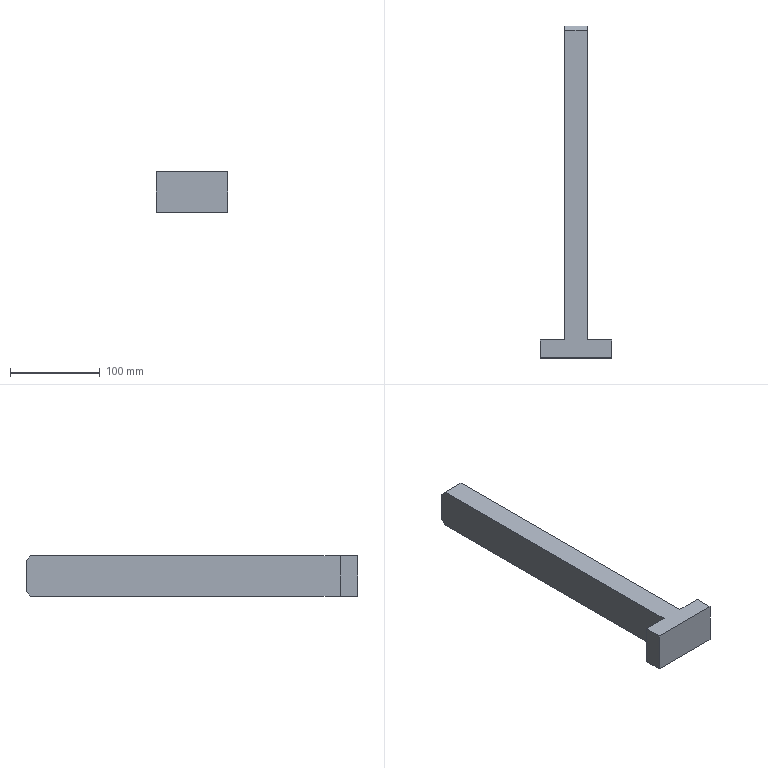Part | STEP file | 2012-06-08-018 | 1 solid | 12 faces | box 80 x 370 x 45 mm | volume 465125 mm3 | plane 12
STEP:
#1=CARTESIAN_POINT('',(0.,0.,0.));
#2=DIRECTION('',(0.,0.,1.));
#3=DIRECTION('',(1.,0.,0.));
#4=AXIS2_PLACEMENT_3D('',#1,#2,#3);
#5=CARTESIAN_POINT('',(0.,20.,0.));
#6=VERTEX_POINT('',#5);
#7=CARTESIAN_POINT('',(0.,0.,0.));
#8=VERTEX_POINT('',#7);
#9=CARTESIAN_POINT('',(0.,0.,0.));
#10=DIRECTION('',(0.,-1.,0.));
#11=VECTOR('',#10,1.);
#12=LINE('',#9,#11);
#13=CARTESIAN_POINT('',(0.,0.,45.));
#14=DIRECTION('',(1.,0.,0.));
#15=DIRECTION('',(0.,0.,-1.));
#16=AXIS2_PLACEMENT_3D('',#13,#14,#15);
#17=PLANE('',#16);
#18=CARTESIAN_POINT('',(45.,0.));
#19=DIRECTION('',(0.,-1.));
#20=VECTOR('',#19,1.);
#21=LINE('',#18,#20);
#22=(GEOMETRIC_REPRESENTATION_CONTEXT(2)PARAMETRIC_REPRESENTATION_CONTEXT()REPRESENTATION_CONTEXT('',''));
#23=DEFINITIONAL_REPRESENTATION('',(#21),#22);
#24=PCURVE('',#17,#23);
#25=CARTESIAN_POINT('',(0.,20.,0.));
#26=DIRECTION('',(0.,0.,-1.));
#27=DIRECTION('',(-1.,0.,0.));
#28=AXIS2_PLACEMENT_3D('',#25,#26,#27);
#29=PLANE('',#28);
#30=CARTESIAN_POINT('',(0.,-20.));
#31=DIRECTION('',(0.,-1.));
#32=VECTOR('',#31,1.);
#33=LINE('',#30,#32);
#34=(GEOMETRIC_REPRESENTATION_CONTEXT(2)PARAMETRIC_REPRESENTATION_CONTEXT()REPRESENTATION_CONTEXT('',''));
#35=DEFINITIONAL_REPRESENTATION('',(#33),#34);
#36=PCURVE('',#29,#35);
#37=SURFACE_CURVE('',#12,(#24,#36),.PCURVE_S1.);
#38=EDGE_CURVE('',#6,#8,#37,.T.);
#39=ORIENTED_EDGE('',*,*,#38,.T.);
#40=CARTESIAN_POINT('',(0.,0.,45.));
#41=VERTEX_POINT('',#40);
#42=CARTESIAN_POINT('',(0.,0.,45.));
#43=DIRECTION('',(0.,0.,-1.));
#44=VECTOR('',#43,1.);
#45=LINE('',#42,#44);
#46=CARTESIAN_POINT('',(0.,0.));
#47=DIRECTION('',(1.,0.));
#48=VECTOR('',#47,1.);
#49=LINE('',#46,#48);
#50=(GEOMETRIC_REPRESENTATION_CONTEXT(2)PARAMETRIC_REPRESENTATION_CONTEXT()REPRESENTATION_CONTEXT('',''));
#51=DEFINITIONAL_REPRESENTATION('',(#49),#50);
#52=PCURVE('',#17,#51);
#53=CARTESIAN_POINT('',(0.,0.,45.));
#54=DIRECTION('',(0.,1.,0.));
#55=DIRECTION('',(0.,0.,1.));
#56=AXIS2_PLACEMENT_3D('',#53,#54,#55);
#57=PLANE('',#56);
#58=CARTESIAN_POINT('',(0.,0.));
#59=DIRECTION('',(-1.,0.));
#60=VECTOR('',#59,1.);
#61=LINE('',#58,#60);
#62=(GEOMETRIC_REPRESENTATION_CONTEXT(2)PARAMETRIC_REPRESENTATION_CONTEXT()REPRESENTATION_CONTEXT('',''));
#63=DEFINITIONAL_REPRESENTATION('',(#61),#62);
#64=PCURVE('',#57,#63);
#65=SURFACE_CURVE('',#45,(#52,#64),.PCURVE_S1.);
#66=EDGE_CURVE('',#41,#8,#65,.T.);
#67=ORIENTED_EDGE('',*,*,#66,.F.);
#68=CARTESIAN_POINT('',(0.,20.,45.));
#69=VERTEX_POINT('',#68);
#70=CARTESIAN_POINT('',(0.,0.,45.));
#71=DIRECTION('',(0.,-1.,0.));
#72=VECTOR('',#71,1.);
#73=LINE('',#70,#72);
#74=CARTESIAN_POINT('',(0.,0.));
#75=DIRECTION('',(0.,-1.));
#76=VECTOR('',#75,1.);
#77=LINE('',#74,#76);
#78=(GEOMETRIC_REPRESENTATION_CONTEXT(2)PARAMETRIC_REPRESENTATION_CONTEXT()REPRESENTATION_CONTEXT('',''));
#79=DEFINITIONAL_REPRESENTATION('',(#77),#78);
#80=PCURVE('',#17,#79);
#81=CARTESIAN_POINT('',(0.,20.,45.));
#82=DIRECTION('',(0.,0.,-1.));
#83=DIRECTION('',(-1.,0.,0.));
#84=AXIS2_PLACEMENT_3D('',#81,#82,#83);
#85=PLANE('',#84);
#86=CARTESIAN_POINT('',(0.,-20.));
#87=DIRECTION('',(0.,-1.));
#88=VECTOR('',#87,1.);
#89=LINE('',#86,#88);
#90=(GEOMETRIC_REPRESENTATION_CONTEXT(2)PARAMETRIC_REPRESENTATION_CONTEXT()REPRESENTATION_CONTEXT('',''));
#91=DEFINITIONAL_REPRESENTATION('',(#89),#90);
#92=PCURVE('',#85,#91);
#93=SURFACE_CURVE('',#73,(#80,#92),.PCURVE_S1.);
#94=EDGE_CURVE('',#69,#41,#93,.T.);
#95=ORIENTED_EDGE('',*,*,#94,.F.);
#96=CARTESIAN_POINT('',(0.,20.,45.));
#97=DIRECTION('',(0.,0.,-1.));
#98=VECTOR('',#97,1.);
#99=LINE('',#96,#98);
#100=CARTESIAN_POINT('',(0.,20.));
#101=DIRECTION('',(1.,0.));
#102=VECTOR('',#101,1.);
#103=LINE('',#100,#102);
#104=(GEOMETRIC_REPRESENTATION_CONTEXT(2)PARAMETRIC_REPRESENTATION_CONTEXT()REPRESENTATION_CONTEXT('',''));
#105=DEFINITIONAL_REPRESENTATION('',(#103),#104);
#106=PCURVE('',#17,#105);
#107=CARTESIAN_POINT('',(0.,20.,45.));
#108=DIRECTION('',(0.,-1.,0.));
#109=DIRECTION('',(1.,0.,0.));
#110=AXIS2_PLACEMENT_3D('',#107,#108,#109);
#111=PLANE('',#110);
#112=CARTESIAN_POINT('',(0.,0.));
#113=DIRECTION('',(0.,-1.));
#114=VECTOR('',#113,1.);
#115=LINE('',#112,#114);
#116=(GEOMETRIC_REPRESENTATION_CONTEXT(2)PARAMETRIC_REPRESENTATION_CONTEXT()REPRESENTATION_CONTEXT('',''));
#117=DEFINITIONAL_REPRESENTATION('',(#115),#116);
#118=PCURVE('',#111,#117);
#119=SURFACE_CURVE('',#99,(#106,#118),.PCURVE_S1.);
#120=EDGE_CURVE('',#69,#6,#119,.T.);
#121=ORIENTED_EDGE('',*,*,#120,.T.);
#122=EDGE_LOOP('',(#39,#67,#95,#121));
#123=FACE_BOUND('',#122,.T.);
#124=ADVANCED_FACE('',(#123),#17,.F.);
#125=CARTESIAN_POINT('',(80.,0.,0.));
#126=VERTEX_POINT('',#125);
#127=CARTESIAN_POINT('',(0.,0.,0.));
#128=DIRECTION('',(1.,0.,0.));
#129=VECTOR('',#128,1.);
#130=LINE('',#127,#129);
#131=CARTESIAN_POINT('',(-45.,0.));
#132=DIRECTION('',(0.,1.));
#133=VECTOR('',#132,1.);
#134=LINE('',#131,#133);
#135=(GEOMETRIC_REPRESENTATION_CONTEXT(2)PARAMETRIC_REPRESENTATION_CONTEXT()REPRESENTATION_CONTEXT('',''));
#136=DEFINITIONAL_REPRESENTATION('',(#134),#135);
#137=PCURVE('',#57,#136);
#138=CARTESIAN_POINT('',(0.,-20.));
#139=DIRECTION('',(-1.,0.));
#140=VECTOR('',#139,1.);
#141=LINE('',#138,#140);
#142=(GEOMETRIC_REPRESENTATION_CONTEXT(2)PARAMETRIC_REPRESENTATION_CONTEXT()REPRESENTATION_CONTEXT('',''));
#143=DEFINITIONAL_REPRESENTATION('',(#141),#142);
#144=PCURVE('',#29,#143);
#145=SURFACE_CURVE('',#130,(#137,#144),.PCURVE_S1.);
#146=EDGE_CURVE('',#8,#126,#145,.T.);
#147=ORIENTED_EDGE('',*,*,#146,.T.);
#148=CARTESIAN_POINT('',(80.,0.,45.));
#149=VERTEX_POINT('',#148);
#150=CARTESIAN_POINT('',(80.,0.,45.));
#151=DIRECTION('',(0.,0.,-1.));
#152=VECTOR('',#151,1.);
#153=LINE('',#150,#152);
#154=CARTESIAN_POINT('',(0.,80.));
#155=DIRECTION('',(-1.,0.));
#156=VECTOR('',#155,1.);
#157=LINE('',#154,#156);
#158=(GEOMETRIC_REPRESENTATION_CONTEXT(2)PARAMETRIC_REPRESENTATION_CONTEXT()REPRESENTATION_CONTEXT('',''));
#159=DEFINITIONAL_REPRESENTATION('',(#157),#158);
#160=PCURVE('',#57,#159);
#161=CARTESIAN_POINT('',(80.,0.,45.));
#162=DIRECTION('',(-1.,0.,0.));
#163=DIRECTION('',(0.,0.,1.));
#164=AXIS2_PLACEMENT_3D('',#161,#162,#163);
#165=PLANE('',#164);
#166=CARTESIAN_POINT('',(0.,0.));
#167=DIRECTION('',(-1.,0.));
#168=VECTOR('',#167,1.);
#169=LINE('',#166,#168);
#170=(GEOMETRIC_REPRESENTATION_CONTEXT(2)PARAMETRIC_REPRESENTATION_CONTEXT()REPRESENTATION_CONTEXT('',''));
#171=DEFINITIONAL_REPRESENTATION('',(#169),#170);
#172=PCURVE('',#165,#171);
#173=SURFACE_CURVE('',#153,(#160,#172),.PCURVE_S1.);
#174=EDGE_CURVE('',#149,#126,#173,.T.);
#175=ORIENTED_EDGE('',*,*,#174,.F.);
#176=CARTESIAN_POINT('',(0.,0.,45.));
#177=DIRECTION('',(1.,0.,0.));
#178=VECTOR('',#177,1.);
#179=LINE('',#176,#178);
#180=CARTESIAN_POINT('',(0.,0.));
#181=DIRECTION('',(0.,1.));
#182=VECTOR('',#181,1.);
#183=LINE('',#180,#182);
#184=(GEOMETRIC_REPRESENTATION_CONTEXT(2)PARAMETRIC_REPRESENTATION_CONTEXT()REPRESENTATION_CONTEXT('',''));
#185=DEFINITIONAL_REPRESENTATION('',(#183),#184);
#186=PCURVE('',#57,#185);
#187=CARTESIAN_POINT('',(0.,-20.));
#188=DIRECTION('',(-1.,0.));
#189=VECTOR('',#188,1.);
#190=LINE('',#187,#189);
#191=(GEOMETRIC_REPRESENTATION_CONTEXT(2)PARAMETRIC_REPRESENTATION_CONTEXT()REPRESENTATION_CONTEXT('',''));
#192=DEFINITIONAL_REPRESENTATION('',(#190),#191);
#193=PCURVE('',#85,#192);
#194=SURFACE_CURVE('',#179,(#186,#193),.PCURVE_S1.);
#195=EDGE_CURVE('',#41,#149,#194,.T.);
#196=ORIENTED_EDGE('',*,*,#195,.F.);
#197=ORIENTED_EDGE('',*,*,#66,.T.);
#198=EDGE_LOOP('',(#147,#175,#196,#197));
#199=FACE_BOUND('',#198,.T.);
#200=ADVANCED_FACE('',(#199),#57,.F.);
#201=CARTESIAN_POINT('',(80.,20.,0.));
#202=VERTEX_POINT('',#201);
#203=CARTESIAN_POINT('',(80.,0.,0.));
#204=DIRECTION('',(0.,1.,0.));
#205=VECTOR('',#204,1.);
#206=LINE('',#203,#205);
#207=CARTESIAN_POINT('',(-45.,0.));
#208=DIRECTION('',(0.,1.));
#209=VECTOR('',#208,1.);
#210=LINE('',#207,#209);
#211=(GEOMETRIC_REPRESENTATION_CONTEXT(2)PARAMETRIC_REPRESENTATION_CONTEXT()REPRESENTATION_CONTEXT('',''));
#212=DEFINITIONAL_REPRESENTATION('',(#210),#211);
#213=PCURVE('',#165,#212);
#214=CARTESIAN_POINT('',(-80.,-20.));
#215=DIRECTION('',(0.,1.));
#216=VECTOR('',#215,1.);
#217=LINE('',#214,#216);
#218=(GEOMETRIC_REPRESENTATION_CONTEXT(2)PARAMETRIC_REPRESENTATION_CONTEXT()REPRESENTATION_CONTEXT('',''));
#219=DEFINITIONAL_REPRESENTATION('',(#217),#218);
#220=PCURVE('',#29,#219);
#221=SURFACE_CURVE('',#206,(#213,#220),.PCURVE_S1.);
#222=EDGE_CURVE('',#126,#202,#221,.T.);
#223=ORIENTED_EDGE('',*,*,#222,.T.);
#224=CARTESIAN_POINT('',(80.,20.,45.));
#225=VERTEX_POINT('',#224);
#226=CARTESIAN_POINT('',(80.,20.,45.));
#227=DIRECTION('',(0.,0.,-1.));
#228=VECTOR('',#227,1.);
#229=LINE('',#226,#228);
#230=CARTESIAN_POINT('',(0.,20.));
#231=DIRECTION('',(-1.,0.));
#232=VECTOR('',#231,1.);
#233=LINE('',#230,#232);
#234=(GEOMETRIC_REPRESENTATION_CONTEXT(2)PARAMETRIC_REPRESENTATION_CONTEXT()REPRESENTATION_CONTEXT('',''));
#235=DEFINITIONAL_REPRESENTATION('',(#233),#234);
#236=PCURVE('',#165,#235);
#237=CARTESIAN_POINT('',(52.5,20.,45.));
#238=DIRECTION('',(0.,-1.,0.));
#239=DIRECTION('',(0.,0.,-1.));
#240=AXIS2_PLACEMENT_3D('',#237,#238,#239);
#241=PLANE('',#240);
#242=CARTESIAN_POINT('',(0.,27.5));
#243=DIRECTION('',(1.,0.));
#244=VECTOR('',#243,1.);
#245=LINE('',#242,#244);
#246=(GEOMETRIC_REPRESENTATION_CONTEXT(2)PARAMETRIC_REPRESENTATION_CONTEXT()REPRESENTATION_CONTEXT('',''));
#247=DEFINITIONAL_REPRESENTATION('',(#245),#246);
#248=PCURVE('',#241,#247);
#249=SURFACE_CURVE('',#229,(#236,#248),.PCURVE_S1.);
#250=EDGE_CURVE('',#225,#202,#249,.T.);
#251=ORIENTED_EDGE('',*,*,#250,.F.);
#252=CARTESIAN_POINT('',(80.,0.,45.));
#253=DIRECTION('',(0.,1.,0.));
#254=VECTOR('',#253,1.);
#255=LINE('',#252,#254);
#256=CARTESIAN_POINT('',(0.,0.));
#257=DIRECTION('',(0.,1.));
#258=VECTOR('',#257,1.);
#259=LINE('',#256,#258);
#260=(GEOMETRIC_REPRESENTATION_CONTEXT(2)PARAMETRIC_REPRESENTATION_CONTEXT()REPRESENTATION_CONTEXT('',''));
#261=DEFINITIONAL_REPRESENTATION('',(#259),#260);
#262=PCURVE('',#165,#261);
#263=CARTESIAN_POINT('',(-80.,-20.));
#264=DIRECTION('',(0.,1.));
#265=VECTOR('',#264,1.);
#266=LINE('',#263,#265);
#267=(GEOMETRIC_REPRESENTATION_CONTEXT(2)PARAMETRIC_REPRESENTATION_CONTEXT()REPRESENTATION_CONTEXT('',''));
#268=DEFINITIONAL_REPRESENTATION('',(#266),#267);
#269=PCURVE('',#85,#268);
#270=SURFACE_CURVE('',#255,(#262,#269),.PCURVE_S1.);
#271=EDGE_CURVE('',#149,#225,#270,.T.);
#272=ORIENTED_EDGE('',*,*,#271,.F.);
#273=ORIENTED_EDGE('',*,*,#174,.T.);
#274=EDGE_LOOP('',(#223,#251,#272,#273));
#275=FACE_BOUND('',#274,.T.);
#276=ADVANCED_FACE('',(#275),#165,.F.);
#277=CARTESIAN_POINT('',(52.5,20.,0.));
#278=VERTEX_POINT('',#277);
#279=CARTESIAN_POINT('',(52.5,20.,0.));
#280=DIRECTION('',(-1.,0.,0.));
#281=VECTOR('',#280,1.);
#282=LINE('',#279,#281);
#283=CARTESIAN_POINT('',(45.,0.));
#284=DIRECTION('',(0.,-1.));
#285=VECTOR('',#284,1.);
#286=LINE('',#283,#285);
#287=(GEOMETRIC_REPRESENTATION_CONTEXT(2)PARAMETRIC_REPRESENTATION_CONTEXT()REPRESENTATION_CONTEXT('',''));
#288=DEFINITIONAL_REPRESENTATION('',(#286),#287);
#289=PCURVE('',#241,#288);
#290=CARTESIAN_POINT('',(-52.5,0.));
#291=DIRECTION('',(1.,0.));
#292=VECTOR('',#291,1.);
#293=LINE('',#290,#292);
#294=(GEOMETRIC_REPRESENTATION_CONTEXT(2)PARAMETRIC_REPRESENTATION_CONTEXT()REPRESENTATION_CONTEXT('',''));
#295=DEFINITIONAL_REPRESENTATION('',(#293),#294);
#296=PCURVE('',#29,#295);
#297=SURFACE_CURVE('',#282,(#289,#296),.PCURVE_S1.);
#298=EDGE_CURVE('',#202,#278,#297,.T.);
#299=ORIENTED_EDGE('',*,*,#298,.T.);
#300=CARTESIAN_POINT('',(52.5,20.,45.));
#301=VERTEX_POINT('',#300);
#302=CARTESIAN_POINT('',(52.5,20.,45.));
#303=DIRECTION('',(0.,0.,-1.));
#304=VECTOR('',#303,1.);
#305=LINE('',#302,#304);
#306=CARTESIAN_POINT('',(0.,0.));
#307=DIRECTION('',(1.,0.));
#308=VECTOR('',#307,1.);
#309=LINE('',#306,#308);
#310=(GEOMETRIC_REPRESENTATION_CONTEXT(2)PARAMETRIC_REPRESENTATION_CONTEXT()REPRESENTATION_CONTEXT('',''));
#311=DEFINITIONAL_REPRESENTATION('',(#309),#310);
#312=PCURVE('',#241,#311);
#313=CARTESIAN_POINT('',(52.5,370.,45.));
#314=DIRECTION('',(-1.,0.,0.));
#315=DIRECTION('',(0.,0.,1.));
#316=AXIS2_PLACEMENT_3D('',#313,#314,#315);
#317=PLANE('',#316);
#318=CARTESIAN_POINT('',(0.,-350.));
#319=DIRECTION('',(-1.,0.));
#320=VECTOR('',#319,1.);
#321=LINE('',#318,#320);
#322=(GEOMETRIC_REPRESENTATION_CONTEXT(2)PARAMETRIC_REPRESENTATION_CONTEXT()REPRESENTATION_CONTEXT('',''));
#323=DEFINITIONAL_REPRESENTATION('',(#321),#322);
#324=PCURVE('',#317,#323);
#325=SURFACE_CURVE('',#305,(#312,#324),.PCURVE_S1.);
#326=EDGE_CURVE('',#301,#278,#325,.T.);
#327=ORIENTED_EDGE('',*,*,#326,.F.);
#328=CARTESIAN_POINT('',(52.5,20.,45.));
#329=DIRECTION('',(-1.,0.,0.));
#330=VECTOR('',#329,1.);
#331=LINE('',#328,#330);
#332=CARTESIAN_POINT('',(0.,0.));
#333=DIRECTION('',(0.,-1.));
#334=VECTOR('',#333,1.);
#335=LINE('',#332,#334);
#336=(GEOMETRIC_REPRESENTATION_CONTEXT(2)PARAMETRIC_REPRESENTATION_CONTEXT()REPRESENTATION_CONTEXT('',''));
#337=DEFINITIONAL_REPRESENTATION('',(#335),#336);
#338=PCURVE('',#241,#337);
#339=CARTESIAN_POINT('',(-52.5,0.));
#340=DIRECTION('',(1.,0.));
#341=VECTOR('',#340,1.);
#342=LINE('',#339,#341);
#343=(GEOMETRIC_REPRESENTATION_CONTEXT(2)PARAMETRIC_REPRESENTATION_CONTEXT()REPRESENTATION_CONTEXT('',''));
#344=DEFINITIONAL_REPRESENTATION('',(#342),#343);
#345=PCURVE('',#85,#344);
#346=SURFACE_CURVE('',#331,(#338,#345),.PCURVE_S1.);
#347=EDGE_CURVE('',#225,#301,#346,.T.);
#348=ORIENTED_EDGE('',*,*,#347,.F.);
#349=ORIENTED_EDGE('',*,*,#250,.T.);
#350=EDGE_LOOP('',(#299,#327,#348,#349));
#351=FACE_BOUND('',#350,.T.);
#352=ADVANCED_FACE('',(#351),#241,.F.);
#353=CARTESIAN_POINT('',(52.5,365.,0.));
#354=VERTEX_POINT('',#353);
#355=CARTESIAN_POINT('',(52.5,370.,0.));
#356=DIRECTION('',(0.,1.,0.));
#357=VECTOR('',#356,1.);
#358=LINE('',#355,#357);
#359=CARTESIAN_POINT('',(-45.,0.));
#360=DIRECTION('',(0.,1.));
#361=VECTOR('',#360,1.);
#362=LINE('',#359,#361);
#363=(GEOMETRIC_REPRESENTATION_CONTEXT(2)PARAMETRIC_REPRESENTATION_CONTEXT()REPRESENTATION_CONTEXT('',''));
#364=DEFINITIONAL_REPRESENTATION('',(#362),#363);
#365=PCURVE('',#317,#364);
#366=CARTESIAN_POINT('',(-52.5,350.));
#367=DIRECTION('',(0.,1.));
#368=VECTOR('',#367,1.);
#369=LINE('',#366,#368);
#370=(GEOMETRIC_REPRESENTATION_CONTEXT(2)PARAMETRIC_REPRESENTATION_CONTEXT()REPRESENTATION_CONTEXT('',''));
#371=DEFINITIONAL_REPRESENTATION('',(#369),#370);
#372=PCURVE('',#29,#371);
#373=SURFACE_CURVE('',#358,(#365,#372),.PCURVE_S1.);
#374=EDGE_CURVE('',#278,#354,#373,.T.);
#375=ORIENTED_EDGE('',*,*,#374,.T.);
#376=CARTESIAN_POINT('',(52.5,370.,5.));
#377=VERTEX_POINT('',#376);
#378=CARTESIAN_POINT('',(52.5,370.,5.));
#379=DIRECTION('',(0.,0.7071,0.7071));
#380=VECTOR('',#379,1.);
#381=LINE('',#378,#380);
#382=CARTESIAN_POINT('',(-40.,0.));
#383=DIRECTION('',(0.7071,0.7071));
#384=VECTOR('',#383,1.);
#385=LINE('',#382,#384);
#386=(GEOMETRIC_REPRESENTATION_CONTEXT(2)PARAMETRIC_REPRESENTATION_CONTEXT()REPRESENTATION_CONTEXT('',''));
#387=DEFINITIONAL_REPRESENTATION('',(#385),#386);
#388=PCURVE('',#317,#387);
#389=CARTESIAN_POINT('',(27.5,370.,5.));
#390=DIRECTION('',(0.,0.7071,-0.7071));
#391=DIRECTION('',(0.,0.7071,0.7071));
#392=AXIS2_PLACEMENT_3D('',#389,#390,#391);
#393=PLANE('',#392);
#394=CARTESIAN_POINT('',(0.,25.));
#395=DIRECTION('',(1.,0.));
#396=VECTOR('',#395,1.);
#397=LINE('',#394,#396);
#398=(GEOMETRIC_REPRESENTATION_CONTEXT(2)PARAMETRIC_REPRESENTATION_CONTEXT()REPRESENTATION_CONTEXT('',''));
#399=DEFINITIONAL_REPRESENTATION('',(#397),#398);
#400=PCURVE('',#393,#399);
#401=SURFACE_CURVE('',#381,(#388,#400),.PCURVE_S1.);
#402=EDGE_CURVE('',#354,#377,#401,.T.);
#403=ORIENTED_EDGE('',*,*,#402,.T.);
#404=CARTESIAN_POINT('',(52.5,370.,40.));
#405=VERTEX_POINT('',#404);
#406=CARTESIAN_POINT('',(52.5,370.,45.));
#407=DIRECTION('',(0.,0.,-1.));
#408=VECTOR('',#407,1.);
#409=LINE('',#406,#408);
#410=CARTESIAN_POINT('',(0.,0.));
#411=DIRECTION('',(-1.,0.));
#412=VECTOR('',#411,1.);
#413=LINE('',#410,#412);
#414=(GEOMETRIC_REPRESENTATION_CONTEXT(2)PARAMETRIC_REPRESENTATION_CONTEXT()REPRESENTATION_CONTEXT('',''));
#415=DEFINITIONAL_REPRESENTATION('',(#413),#414);
#416=PCURVE('',#317,#415);
#417=CARTESIAN_POINT('',(27.5,370.,45.));
#418=DIRECTION('',(0.,-1.,0.));
#419=DIRECTION('',(0.,0.,-1.));
#420=AXIS2_PLACEMENT_3D('',#417,#418,#419);
#421=PLANE('',#420);
#422=CARTESIAN_POINT('',(0.,25.));
#423=DIRECTION('',(1.,0.));
#424=VECTOR('',#423,1.);
#425=LINE('',#422,#424);
#426=(GEOMETRIC_REPRESENTATION_CONTEXT(2)PARAMETRIC_REPRESENTATION_CONTEXT()REPRESENTATION_CONTEXT('',''));
#427=DEFINITIONAL_REPRESENTATION('',(#425),#426);
#428=PCURVE('',#421,#427);
#429=SURFACE_CURVE('',#409,(#416,#428),.PCURVE_S1.);
#430=EDGE_CURVE('',#405,#377,#429,.T.);
#431=ORIENTED_EDGE('',*,*,#430,.F.);
#432=CARTESIAN_POINT('',(52.5,365.,45.));
#433=VERTEX_POINT('',#432);
#434=CARTESIAN_POINT('',(52.5,365.,45.));
#435=DIRECTION('',(0.,-0.7071,0.7071));
#436=VECTOR('',#435,1.);
#437=LINE('',#434,#436);
#438=CARTESIAN_POINT('',(0.,-5.));
#439=DIRECTION('',(0.7071,-0.7071));
#440=VECTOR('',#439,1.);
#441=LINE('',#438,#440);
#442=(GEOMETRIC_REPRESENTATION_CONTEXT(2)PARAMETRIC_REPRESENTATION_CONTEXT()REPRESENTATION_CONTEXT('',''));
#443=DEFINITIONAL_REPRESENTATION('',(#441),#442);
#444=PCURVE('',#317,#443);
#445=CARTESIAN_POINT('',(0.,365.,45.));
#446=DIRECTION('',(0.,-0.7071,-0.7071));
#447=DIRECTION('',(0.,0.7071,-0.7071));
#448=AXIS2_PLACEMENT_3D('',#445,#446,#447);
#449=PLANE('',#448);
#450=CARTESIAN_POINT('',(0.,52.5));
#451=DIRECTION('',(-1.,0.));
#452=VECTOR('',#451,1.);
#453=LINE('',#450,#452);
#454=(GEOMETRIC_REPRESENTATION_CONTEXT(2)PARAMETRIC_REPRESENTATION_CONTEXT()REPRESENTATION_CONTEXT('',''));
#455=DEFINITIONAL_REPRESENTATION('',(#453),#454);
#456=PCURVE('',#449,#455);
#457=SURFACE_CURVE('',#437,(#444,#456),.PCURVE_S1.);
#458=EDGE_CURVE('',#405,#433,#457,.T.);
#459=ORIENTED_EDGE('',*,*,#458,.T.);
#460=CARTESIAN_POINT('',(52.5,370.,45.));
#461=DIRECTION('',(0.,1.,0.));
#462=VECTOR('',#461,1.);
#463=LINE('',#460,#462);
#464=CARTESIAN_POINT('',(0.,0.));
#465=DIRECTION('',(0.,1.));
#466=VECTOR('',#465,1.);
#467=LINE('',#464,#466);
#468=(GEOMETRIC_REPRESENTATION_CONTEXT(2)PARAMETRIC_REPRESENTATION_CONTEXT()REPRESENTATION_CONTEXT('',''));
#469=DEFINITIONAL_REPRESENTATION('',(#467),#468);
#470=PCURVE('',#317,#469);
#471=CARTESIAN_POINT('',(-52.5,350.));
#472=DIRECTION('',(0.,1.));
#473=VECTOR('',#472,1.);
#474=LINE('',#471,#473);
#475=(GEOMETRIC_REPRESENTATION_CONTEXT(2)PARAMETRIC_REPRESENTATION_CONTEXT()REPRESENTATION_CONTEXT('',''));
#476=DEFINITIONAL_REPRESENTATION('',(#474),#475);
#477=PCURVE('',#85,#476);
#478=SURFACE_CURVE('',#463,(#470,#477),.PCURVE_S1.);
#479=EDGE_CURVE('',#301,#433,#478,.T.);
#480=ORIENTED_EDGE('',*,*,#479,.F.);
#481=ORIENTED_EDGE('',*,*,#326,.T.);
#482=EDGE_LOOP('',(#375,#403,#431,#459,#480,#481));
#483=FACE_BOUND('',#482,.T.);
#484=ADVANCED_FACE('',(#483),#317,.F.);
#485=ORIENTED_EDGE('',*,*,#430,.T.);
#486=CARTESIAN_POINT('',(27.5,370.,5.));
#487=VERTEX_POINT('',#486);
#488=CARTESIAN_POINT('',(27.5,370.,5.));
#489=DIRECTION('',(-1.,0.,0.));
#490=VECTOR('',#489,1.);
#491=LINE('',#488,#490);
#492=CARTESIAN_POINT('',(40.,0.));
#493=DIRECTION('',(0.,-1.));
#494=VECTOR('',#493,1.);
#495=LINE('',#492,#494);
#496=(GEOMETRIC_REPRESENTATION_CONTEXT(2)PARAMETRIC_REPRESENTATION_CONTEXT()REPRESENTATION_CONTEXT('',''));
#497=DEFINITIONAL_REPRESENTATION('',(#495),#496);
#498=PCURVE('',#421,#497);
#499=CARTESIAN_POINT('',(0.,0.));
#500=DIRECTION('',(0.,-1.));
#501=VECTOR('',#500,1.);
#502=LINE('',#499,#501);
#503=(GEOMETRIC_REPRESENTATION_CONTEXT(2)PARAMETRIC_REPRESENTATION_CONTEXT()REPRESENTATION_CONTEXT('',''));
#504=DEFINITIONAL_REPRESENTATION('',(#502),#503);
#505=PCURVE('',#393,#504);
#506=SURFACE_CURVE('',#491,(#498,#505),.PCURVE_S1.);
#507=EDGE_CURVE('',#377,#487,#506,.T.);
#508=ORIENTED_EDGE('',*,*,#507,.T.);
#509=CARTESIAN_POINT('',(27.5,370.,40.));
#510=VERTEX_POINT('',#509);
#511=CARTESIAN_POINT('',(27.5,370.,45.));
#512=DIRECTION('',(0.,0.,-1.));
#513=VECTOR('',#512,1.);
#514=LINE('',#511,#513);
#515=CARTESIAN_POINT('',(0.,0.));
#516=DIRECTION('',(1.,0.));
#517=VECTOR('',#516,1.);
#518=LINE('',#515,#517);
#519=(GEOMETRIC_REPRESENTATION_CONTEXT(2)PARAMETRIC_REPRESENTATION_CONTEXT()REPRESENTATION_CONTEXT('',''));
#520=DEFINITIONAL_REPRESENTATION('',(#518),#519);
#521=PCURVE('',#421,#520);
#522=CARTESIAN_POINT('',(27.5,20.,45.));
#523=DIRECTION('',(1.,0.,0.));
#524=DIRECTION('',(0.,1.,0.));
#525=AXIS2_PLACEMENT_3D('',#522,#523,#524);
#526=PLANE('',#525);
#527=CARTESIAN_POINT('',(350.,0.));
#528=DIRECTION('',(0.,-1.));
#529=VECTOR('',#528,1.);
#530=LINE('',#527,#529);
#531=(GEOMETRIC_REPRESENTATION_CONTEXT(2)PARAMETRIC_REPRESENTATION_CONTEXT()REPRESENTATION_CONTEXT('',''));
#532=DEFINITIONAL_REPRESENTATION('',(#530),#531);
#533=PCURVE('',#526,#532);
#534=SURFACE_CURVE('',#514,(#521,#533),.PCURVE_S1.);
#535=EDGE_CURVE('',#510,#487,#534,.T.);
#536=ORIENTED_EDGE('',*,*,#535,.F.);
#537=CARTESIAN_POINT('',(27.5,370.,40.));
#538=DIRECTION('',(1.,0.,0.));
#539=VECTOR('',#538,1.);
#540=LINE('',#537,#539);
#541=CARTESIAN_POINT('',(5.,0.));
#542=DIRECTION('',(0.,1.));
#543=VECTOR('',#542,1.);
#544=LINE('',#541,#543);
#545=(GEOMETRIC_REPRESENTATION_CONTEXT(2)PARAMETRIC_REPRESENTATION_CONTEXT()REPRESENTATION_CONTEXT('',''));
#546=DEFINITIONAL_REPRESENTATION('',(#544),#545);
#547=PCURVE('',#421,#546);
#548=CARTESIAN_POINT('',(7.071,27.5));
#549=DIRECTION('',(0.,1.));
#550=VECTOR('',#549,1.);
#551=LINE('',#548,#550);
#552=(GEOMETRIC_REPRESENTATION_CONTEXT(2)PARAMETRIC_REPRESENTATION_CONTEXT()REPRESENTATION_CONTEXT('',''));
#553=DEFINITIONAL_REPRESENTATION('',(#551),#552);
#554=PCURVE('',#449,#553);
#555=SURFACE_CURVE('',#540,(#547,#554),.PCURVE_S1.);
#556=EDGE_CURVE('',#510,#405,#555,.T.);
#557=ORIENTED_EDGE('',*,*,#556,.T.);
#558=EDGE_LOOP('',(#485,#508,#536,#557));
#559=FACE_BOUND('',#558,.T.);
#560=ADVANCED_FACE('',(#559),#421,.F.);
#561=ORIENTED_EDGE('',*,*,#535,.T.);
#562=CARTESIAN_POINT('',(27.5,365.,0.));
#563=VERTEX_POINT('',#562);
#564=CARTESIAN_POINT('',(27.5,370.,5.));
#565=DIRECTION('',(0.,-0.7071,-0.7071));
#566=VECTOR('',#565,1.);
#567=LINE('',#564,#566);
#568=CARTESIAN_POINT('',(350.,-40.));
#569=DIRECTION('',(-0.7071,-0.7071));
#570=VECTOR('',#569,1.);
#571=LINE('',#568,#570);
#572=(GEOMETRIC_REPRESENTATION_CONTEXT(2)PARAMETRIC_REPRESENTATION_CONTEXT()REPRESENTATION_CONTEXT('',''));
#573=DEFINITIONAL_REPRESENTATION('',(#571),#572);
#574=PCURVE('',#526,#573);
#575=CARTESIAN_POINT('',(0.,0.));
#576=DIRECTION('',(-1.,0.));
#577=VECTOR('',#576,1.);
#578=LINE('',#575,#577);
#579=(GEOMETRIC_REPRESENTATION_CONTEXT(2)PARAMETRIC_REPRESENTATION_CONTEXT()REPRESENTATION_CONTEXT('',''));
#580=DEFINITIONAL_REPRESENTATION('',(#578),#579);
#581=PCURVE('',#393,#580);
#582=SURFACE_CURVE('',#567,(#574,#581),.PCURVE_S1.);
#583=EDGE_CURVE('',#487,#563,#582,.T.);
#584=ORIENTED_EDGE('',*,*,#583,.T.);
#585=CARTESIAN_POINT('',(27.5,20.,0.));
#586=VERTEX_POINT('',#585);
#587=CARTESIAN_POINT('',(27.5,20.,0.));
#588=DIRECTION('',(0.,-1.,0.));
#589=VECTOR('',#588,1.);
#590=LINE('',#587,#589);
#591=CARTESIAN_POINT('',(0.,-45.));
#592=DIRECTION('',(-1.,0.));
#593=VECTOR('',#592,1.);
#594=LINE('',#591,#593);
#595=(GEOMETRIC_REPRESENTATION_CONTEXT(2)PARAMETRIC_REPRESENTATION_CONTEXT()REPRESENTATION_CONTEXT('',''));
#596=DEFINITIONAL_REPRESENTATION('',(#594),#595);
#597=PCURVE('',#526,#596);
#598=CARTESIAN_POINT('',(-27.5,0.));
#599=DIRECTION('',(0.,-1.));
#600=VECTOR('',#599,1.);
#601=LINE('',#598,#600);
#602=(GEOMETRIC_REPRESENTATION_CONTEXT(2)PARAMETRIC_REPRESENTATION_CONTEXT()REPRESENTATION_CONTEXT('',''));
#603=DEFINITIONAL_REPRESENTATION('',(#601),#602);
#604=PCURVE('',#29,#603);
#605=SURFACE_CURVE('',#590,(#597,#604),.PCURVE_S1.);
#606=EDGE_CURVE('',#563,#586,#605,.T.);
#607=ORIENTED_EDGE('',*,*,#606,.T.);
#608=CARTESIAN_POINT('',(27.5,20.,45.));
#609=VERTEX_POINT('',#608);
#610=CARTESIAN_POINT('',(27.5,20.,45.));
#611=DIRECTION('',(0.,0.,-1.));
#612=VECTOR('',#611,1.);
#613=LINE('',#610,#612);
#614=CARTESIAN_POINT('',(0.,0.));
#615=DIRECTION('',(0.,-1.));
#616=VECTOR('',#615,1.);
#617=LINE('',#614,#616);
#618=(GEOMETRIC_REPRESENTATION_CONTEXT(2)PARAMETRIC_REPRESENTATION_CONTEXT()REPRESENTATION_CONTEXT('',''));
#619=DEFINITIONAL_REPRESENTATION('',(#617),#618);
#620=PCURVE('',#526,#619);
#621=CARTESIAN_POINT('',(27.5,0.));
#622=DIRECTION('',(0.,-1.));
#623=VECTOR('',#622,1.);
#624=LINE('',#621,#623);
#625=(GEOMETRIC_REPRESENTATION_CONTEXT(2)PARAMETRIC_REPRESENTATION_CONTEXT()REPRESENTATION_CONTEXT('',''));
#626=DEFINITIONAL_REPRESENTATION('',(#624),#625);
#627=PCURVE('',#111,#626);
#628=SURFACE_CURVE('',#613,(#620,#627),.PCURVE_S1.);
#629=EDGE_CURVE('',#609,#586,#628,.T.);
#630=ORIENTED_EDGE('',*,*,#629,.F.);
#631=CARTESIAN_POINT('',(27.5,365.,45.));
#632=VERTEX_POINT('',#631);
#633=CARTESIAN_POINT('',(27.5,20.,45.));
#634=DIRECTION('',(0.,-1.,0.));
#635=VECTOR('',#634,1.);
#636=LINE('',#633,#635);
#637=CARTESIAN_POINT('',(0.,0.));
#638=DIRECTION('',(-1.,0.));
#639=VECTOR('',#638,1.);
#640=LINE('',#637,#639);
#641=(GEOMETRIC_REPRESENTATION_CONTEXT(2)PARAMETRIC_REPRESENTATION_CONTEXT()REPRESENTATION_CONTEXT('',''));
#642=DEFINITIONAL_REPRESENTATION('',(#640),#641);
#643=PCURVE('',#526,#642);
#644=CARTESIAN_POINT('',(-27.5,0.));
#645=DIRECTION('',(0.,-1.));
#646=VECTOR('',#645,1.);
#647=LINE('',#644,#646);
#648=(GEOMETRIC_REPRESENTATION_CONTEXT(2)PARAMETRIC_REPRESENTATION_CONTEXT()REPRESENTATION_CONTEXT('',''));
#649=DEFINITIONAL_REPRESENTATION('',(#647),#648);
#650=PCURVE('',#85,#649);
#651=SURFACE_CURVE('',#636,(#643,#650),.PCURVE_S1.);
#652=EDGE_CURVE('',#632,#609,#651,.T.);
#653=ORIENTED_EDGE('',*,*,#652,.F.);
#654=CARTESIAN_POINT('',(27.5,365.,45.));
#655=DIRECTION('',(0.,0.7071,-0.7071));
#656=VECTOR('',#655,1.);
#657=LINE('',#654,#656);
#658=CARTESIAN_POINT('',(345.,0.));
#659=DIRECTION('',(0.7071,-0.7071));
#660=VECTOR('',#659,1.);
#661=LINE('',#658,#660);
#662=(GEOMETRIC_REPRESENTATION_CONTEXT(2)PARAMETRIC_REPRESENTATION_CONTEXT()REPRESENTATION_CONTEXT('',''));
#663=DEFINITIONAL_REPRESENTATION('',(#661),#662);
#664=PCURVE('',#526,#663);
#665=CARTESIAN_POINT('',(0.,27.5));
#666=DIRECTION('',(1.,0.));
#667=VECTOR('',#666,1.);
#668=LINE('',#665,#667);
#669=(GEOMETRIC_REPRESENTATION_CONTEXT(2)PARAMETRIC_REPRESENTATION_CONTEXT()REPRESENTATION_CONTEXT('',''));
#670=DEFINITIONAL_REPRESENTATION('',(#668),#669);
#671=PCURVE('',#449,#670);
#672=SURFACE_CURVE('',#657,(#664,#671),.PCURVE_S1.);
#673=EDGE_CURVE('',#632,#510,#672,.T.);
#674=ORIENTED_EDGE('',*,*,#673,.T.);
#675=EDGE_LOOP('',(#561,#584,#607,#630,#653,#674));
#676=FACE_BOUND('',#675,.T.);
#677=ADVANCED_FACE('',(#676),#526,.F.);
#678=CARTESIAN_POINT('',(0.,20.,0.));
#679=DIRECTION('',(-1.,0.,0.));
#680=VECTOR('',#679,1.);
#681=LINE('',#678,#680);
#682=CARTESIAN_POINT('',(0.,-45.));
#683=DIRECTION('',(-1.,0.));
#684=VECTOR('',#683,1.);
#685=LINE('',#682,#684);
#686=(GEOMETRIC_REPRESENTATION_CONTEXT(2)PARAMETRIC_REPRESENTATION_CONTEXT()REPRESENTATION_CONTEXT('',''));
#687=DEFINITIONAL_REPRESENTATION('',(#685),#686);
#688=PCURVE('',#111,#687);
#689=CARTESIAN_POINT('',(0.,0.));
#690=DIRECTION('',(1.,0.));
#691=VECTOR('',#690,1.);
#692=LINE('',#689,#691);
#693=(GEOMETRIC_REPRESENTATION_CONTEXT(2)PARAMETRIC_REPRESENTATION_CONTEXT()REPRESENTATION_CONTEXT('',''));
#694=DEFINITIONAL_REPRESENTATION('',(#692),#693);
#695=PCURVE('',#29,#694);
#696=SURFACE_CURVE('',#681,(#688,#695),.PCURVE_S1.);
#697=EDGE_CURVE('',#586,#6,#696,.T.);
#698=ORIENTED_EDGE('',*,*,#697,.T.);
#699=ORIENTED_EDGE('',*,*,#120,.F.);
#700=CARTESIAN_POINT('',(0.,20.,45.));
#701=DIRECTION('',(-1.,0.,0.));
#702=VECTOR('',#701,1.);
#703=LINE('',#700,#702);
#704=CARTESIAN_POINT('',(0.,0.));
#705=DIRECTION('',(-1.,0.));
#706=VECTOR('',#705,1.);
#707=LINE('',#704,#706);
#708=(GEOMETRIC_REPRESENTATION_CONTEXT(2)PARAMETRIC_REPRESENTATION_CONTEXT()REPRESENTATION_CONTEXT('',''));
#709=DEFINITIONAL_REPRESENTATION('',(#707),#708);
#710=PCURVE('',#111,#709);
#711=CARTESIAN_POINT('',(0.,0.));
#712=DIRECTION('',(1.,0.));
#713=VECTOR('',#712,1.);
#714=LINE('',#711,#713);
#715=(GEOMETRIC_REPRESENTATION_CONTEXT(2)PARAMETRIC_REPRESENTATION_CONTEXT()REPRESENTATION_CONTEXT('',''));
#716=DEFINITIONAL_REPRESENTATION('',(#714),#715);
#717=PCURVE('',#85,#716);
#718=SURFACE_CURVE('',#703,(#710,#717),.PCURVE_S1.);
#719=EDGE_CURVE('',#609,#69,#718,.T.);
#720=ORIENTED_EDGE('',*,*,#719,.F.);
#721=ORIENTED_EDGE('',*,*,#629,.T.);
#722=EDGE_LOOP('',(#698,#699,#720,#721));
#723=FACE_BOUND('',#722,.T.);
#724=ADVANCED_FACE('',(#723),#111,.F.);
#725=ORIENTED_EDGE('',*,*,#479,.T.);
#726=CARTESIAN_POINT('',(0.,365.,45.));
#727=DIRECTION('',(-1.,0.,0.));
#728=VECTOR('',#727,1.);
#729=LINE('',#726,#728);
#730=CARTESIAN_POINT('',(0.,345.));
#731=DIRECTION('',(1.,0.));
#732=VECTOR('',#731,1.);
#733=LINE('',#730,#732);
#734=(GEOMETRIC_REPRESENTATION_CONTEXT(2)PARAMETRIC_REPRESENTATION_CONTEXT()REPRESENTATION_CONTEXT('',''));
#735=DEFINITIONAL_REPRESENTATION('',(#733),#734);
#736=PCURVE('',#85,#735);
#737=CARTESIAN_POINT('',(0.,0.));
#738=DIRECTION('',(0.,-1.));
#739=VECTOR('',#738,1.);
#740=LINE('',#737,#739);
#741=(GEOMETRIC_REPRESENTATION_CONTEXT(2)PARAMETRIC_REPRESENTATION_CONTEXT()REPRESENTATION_CONTEXT('',''));
#742=DEFINITIONAL_REPRESENTATION('',(#740),#741);
#743=PCURVE('',#449,#742);
#744=SURFACE_CURVE('',#729,(#736,#743),.PCURVE_S1.);
#745=EDGE_CURVE('',#433,#632,#744,.T.);
#746=ORIENTED_EDGE('',*,*,#745,.T.);
#747=ORIENTED_EDGE('',*,*,#652,.T.);
#748=ORIENTED_EDGE('',*,*,#719,.T.);
#749=ORIENTED_EDGE('',*,*,#94,.T.);
#750=ORIENTED_EDGE('',*,*,#195,.T.);
#751=ORIENTED_EDGE('',*,*,#271,.T.);
#752=ORIENTED_EDGE('',*,*,#347,.T.);
#753=EDGE_LOOP('',(#725,#746,#747,#748,#749,#750,#751,#752));
#754=FACE_BOUND('',#753,.T.);
#755=ADVANCED_FACE('',(#754),#85,.F.);
#756=ORIENTED_EDGE('',*,*,#606,.F.);
#757=CARTESIAN_POINT('',(52.5,365.,0.));
#758=DIRECTION('',(1.,0.,0.));
#759=VECTOR('',#758,1.);
#760=LINE('',#757,#759);
#761=CARTESIAN_POINT('',(-52.5,345.));
#762=DIRECTION('',(-1.,0.));
#763=VECTOR('',#762,1.);
#764=LINE('',#761,#763);
#765=(GEOMETRIC_REPRESENTATION_CONTEXT(2)PARAMETRIC_REPRESENTATION_CONTEXT()REPRESENTATION_CONTEXT('',''));
#766=DEFINITIONAL_REPRESENTATION('',(#764),#765);
#767=PCURVE('',#29,#766);
#768=CARTESIAN_POINT('',(-7.071,25.));
#769=DIRECTION('',(0.,1.));
#770=VECTOR('',#769,1.);
#771=LINE('',#768,#770);
#772=(GEOMETRIC_REPRESENTATION_CONTEXT(2)PARAMETRIC_REPRESENTATION_CONTEXT()REPRESENTATION_CONTEXT('',''));
#773=DEFINITIONAL_REPRESENTATION('',(#771),#772);
#774=PCURVE('',#393,#773);
#775=SURFACE_CURVE('',#760,(#767,#774),.PCURVE_S1.);
#776=EDGE_CURVE('',#563,#354,#775,.T.);
#777=ORIENTED_EDGE('',*,*,#776,.T.);
#778=ORIENTED_EDGE('',*,*,#374,.F.);
#779=ORIENTED_EDGE('',*,*,#298,.F.);
#780=ORIENTED_EDGE('',*,*,#222,.F.);
#781=ORIENTED_EDGE('',*,*,#146,.F.);
#782=ORIENTED_EDGE('',*,*,#38,.F.);
#783=ORIENTED_EDGE('',*,*,#697,.F.);
#784=EDGE_LOOP('',(#756,#777,#778,#779,#780,#781,#782,#783));
#785=FACE_BOUND('',#784,.T.);
#786=ADVANCED_FACE('',(#785),#29,.T.);
#787=ORIENTED_EDGE('',*,*,#402,.F.);
#788=ORIENTED_EDGE('',*,*,#776,.F.);
#789=ORIENTED_EDGE('',*,*,#583,.F.);
#790=ORIENTED_EDGE('',*,*,#507,.F.);
#791=EDGE_LOOP('',(#787,#788,#789,#790));
#792=FACE_BOUND('',#791,.T.);
#793=ADVANCED_FACE('',(#792),#393,.T.);
#794=ORIENTED_EDGE('',*,*,#458,.F.);
#795=ORIENTED_EDGE('',*,*,#556,.F.);
#796=ORIENTED_EDGE('',*,*,#673,.F.);
#797=ORIENTED_EDGE('',*,*,#745,.F.);
#798=EDGE_LOOP('',(#794,#795,#796,#797));
#799=FACE_BOUND('',#798,.T.);
#800=ADVANCED_FACE('',(#799),#449,.F.);
#801=CLOSED_SHELL('',(#124,#200,#276,#352,#484,#560,#677,#724,#755,#786,#793,#800));
#802=MANIFOLD_SOLID_BREP('',#801);
#803=(LENGTH_UNIT()NAMED_UNIT(*)SI_UNIT(.MILLI.,.METRE.));
#804=UNCERTAINTY_MEASURE_WITH_UNIT(LENGTH_MEASURE(0.0000001),#803,'','');
#805=(NAMED_UNIT(*)PLANE_ANGLE_UNIT()SI_UNIT($,.RADIAN.));
#806=(NAMED_UNIT(*)SI_UNIT($,.STERADIAN.)SOLID_ANGLE_UNIT());
#807=(GEOMETRIC_REPRESENTATION_CONTEXT(3)GLOBAL_UNCERTAINTY_ASSIGNED_CONTEXT((#804))GLOBAL_UNIT_ASSIGNED_CONTEXT((#803,#805,#806))REPRESENTATION_CONTEXT('',''));
#808=ADVANCED_BREP_SHAPE_REPRESENTATION('',(#4,#802),#807);